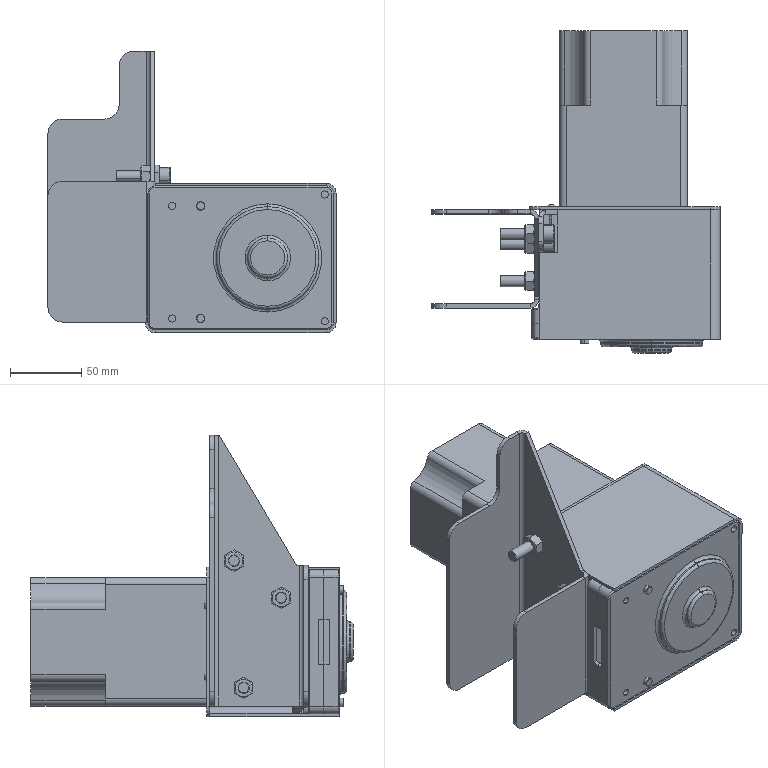Part | SolidWorks | 25 solids | 843 faces | box 202.23 x 226 x 197.5 mm | volume 1360505 mm3 | plane 446 | cylinder 252 | cone 92 | torus 42 | spline 7 | sphere 4 | commonest cylinder face diameters 10 x55 7 x29 6 x22 8 x22 13 x14 20 x14